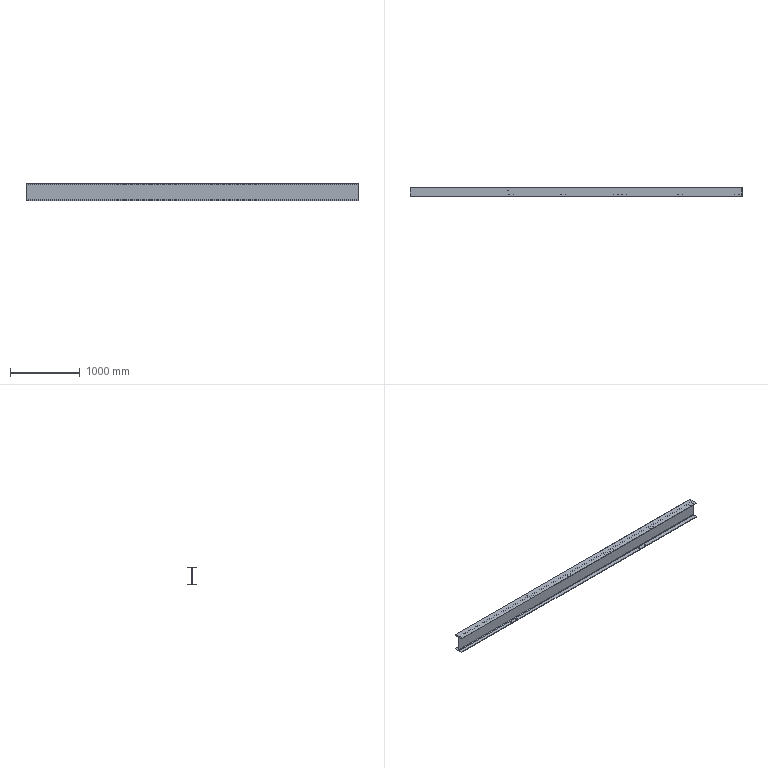Part | STEP file | PN_0038 main beam HN250X125=5225_Default<As Machined> | 1 solid | 41 faces | box 4770 x 125 x 250 mm | volume 17605699 mm3 | cylinder 25 | plane 16 | commonest cylinder face diameters 6.8 x13 18 x8 16 x4